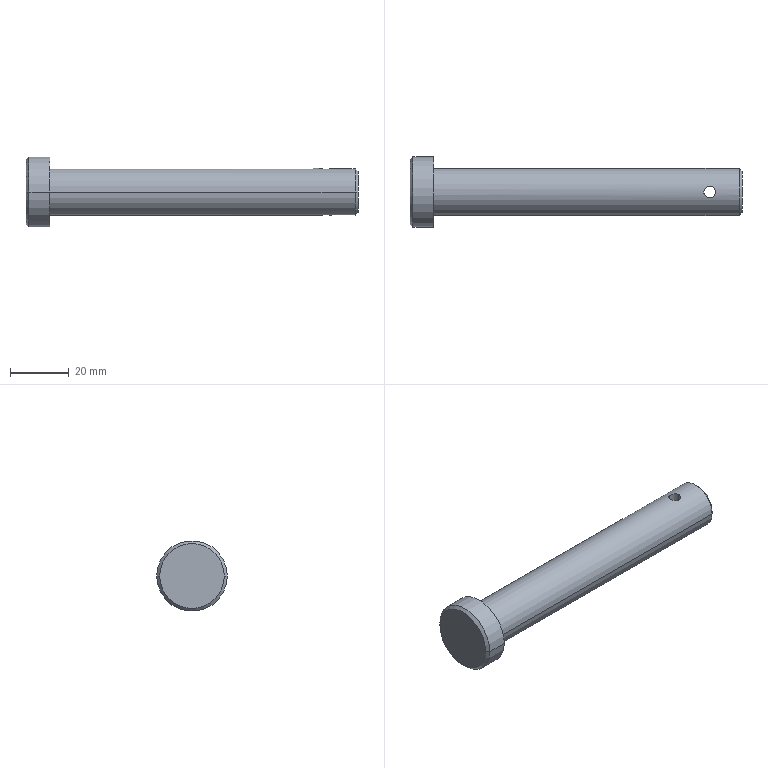Part | SolidWorks | features Chamfer 2, ICE 1, Revolution 1 | 1 solid | 13 faces | box 113 x 24 x 24 mm | volume 24470 mm3 | cylinder 6 | cone 4 | plane 3 | commonest cylinder face diameters 4 x2 16 x2 24 x2
STEP:
#1=CARTESIAN_POINT('',(-113.,-11.,0.));
#2=VERTEX_POINT('',#1);
#3=CARTESIAN_POINT('',(-113.,11.,0.));
#4=VERTEX_POINT('',#3);
#5=CARTESIAN_POINT('',(-113.,0.,0.));
#6=DIRECTION('',(-1.,0.,0.));
#7=DIRECTION('',(0.,-1.,0.));
#8=AXIS2_PLACEMENT_3D('',#5,#6,#7);
#9=CIRCLE('',#8,11.);
#10=EDGE_CURVE('',#2,#4,#9,.T.);
#11=ORIENTED_EDGE('',*,*,#10,.F.);
#12=CARTESIAN_POINT('',(-112.,-12.,0.));
#13=VERTEX_POINT('',#12);
#14=CARTESIAN_POINT('',(-112.,-12.,0.));
#15=DIRECTION('',(0.7071,-0.7071,0.));
#16=VECTOR('',#15,1000.);
#17=LINE('',#14,#16);
#18=EDGE_CURVE('',#2,#13,#17,.T.);
#19=ORIENTED_EDGE('',*,*,#18,.T.);
#20=CARTESIAN_POINT('',(-112.,12.,0.));
#21=VERTEX_POINT('',#20);
#22=CARTESIAN_POINT('',(-112.,0.,0.));
#23=DIRECTION('',(1.,0.,0.));
#24=DIRECTION('',(0.,-1.,0.));
#25=AXIS2_PLACEMENT_3D('',#22,#23,#24);
#26=CIRCLE('',#25,12.);
#27=EDGE_CURVE('',#21,#13,#26,.T.);
#28=ORIENTED_EDGE('',*,*,#27,.F.);
#29=CARTESIAN_POINT('',(-112.,12.,0.));
#30=DIRECTION('',(0.7071,0.7071,0.));
#31=VECTOR('',#30,1000.);
#32=LINE('',#29,#31);
#33=EDGE_CURVE('',#4,#21,#32,.T.);
#34=ORIENTED_EDGE('',*,*,#33,.F.);
#35=EDGE_LOOP('',(#11,#19,#28,#34));
#36=FACE_OUTER_BOUND('',#35,.T.);
#37=CARTESIAN_POINT('',(-112.,0.,0.));
#38=DIRECTION('',(1.,0.,0.));
#39=DIRECTION('',(0.,1.,0.));
#40=AXIS2_PLACEMENT_3D('',#37,#38,#39);
#41=CONICAL_SURFACE('',#40,12.,0.7854);
#42=ADVANCED_FACE('',(#36),#41,.T.);
#43=CARTESIAN_POINT('',(0.,7.,0.));
#44=VERTEX_POINT('',#43);
#45=CARTESIAN_POINT('',(0.,-7.,0.));
#46=VERTEX_POINT('',#45);
#47=CARTESIAN_POINT('',(0.,0.,0.));
#48=DIRECTION('',(1.,0.,0.));
#49=DIRECTION('',(0.,1.,0.));
#50=AXIS2_PLACEMENT_3D('',#47,#48,#49);
#51=CIRCLE('',#50,7.);
#52=EDGE_CURVE('',#44,#46,#51,.T.);
#53=ORIENTED_EDGE('',*,*,#52,.F.);
#54=CARTESIAN_POINT('',(-1.,8.,0.));
#55=VERTEX_POINT('',#54);
#56=CARTESIAN_POINT('',(0.,7.,0.));
#57=DIRECTION('',(-0.7071,0.7071,0.));
#58=VECTOR('',#57,1000.);
#59=LINE('',#56,#58);
#60=EDGE_CURVE('',#44,#55,#59,.T.);
#61=ORIENTED_EDGE('',*,*,#60,.T.);
#62=CARTESIAN_POINT('',(-1.,-8.,0.));
#63=VERTEX_POINT('',#62);
#64=CARTESIAN_POINT('',(-1.,0.,0.));
#65=DIRECTION('',(-1.,0.,0.));
#66=DIRECTION('',(0.,1.,0.));
#67=AXIS2_PLACEMENT_3D('',#64,#65,#66);
#68=CIRCLE('',#67,8.);
#69=EDGE_CURVE('',#63,#55,#68,.T.);
#70=ORIENTED_EDGE('',*,*,#69,.F.);
#71=CARTESIAN_POINT('',(0.,-7.,0.));
#72=DIRECTION('',(-0.7071,-0.7071,0.));
#73=VECTOR('',#72,1000.);
#74=LINE('',#71,#73);
#75=EDGE_CURVE('',#46,#63,#74,.T.);
#76=ORIENTED_EDGE('',*,*,#75,.F.);
#77=EDGE_LOOP('',(#53,#61,#70,#76));
#78=FACE_OUTER_BOUND('',#77,.T.);
#79=CARTESIAN_POINT('',(0.,0.,0.));
#80=DIRECTION('',(-1.,0.,0.));
#81=DIRECTION('',(0.,-1.,0.));
#82=AXIS2_PLACEMENT_3D('',#79,#80,#81);
#83=CONICAL_SURFACE('',#82,7.,0.7854);
#84=ADVANCED_FACE('',(#78),#83,.T.);
#85=CARTESIAN_POINT('',(-9.,0.,-8.));
#86=VERTEX_POINT('',#85);
#87=CARTESIAN_POINT('',(-13.,0.,-8.));
#88=VERTEX_POINT('',#87);
#89=CARTESIAN_POINT('',(-9.,0.,-8.));
#90=CARTESIAN_POINT('',(-9.,-0.1327,-8.));
#91=CARTESIAN_POINT('',(-9.013,-0.2631,-7.997));
#92=CARTESIAN_POINT('',(-9.064,-0.5195,-7.984));
#93=CARTESIAN_POINT('',(-9.103,-0.6468,-7.975));
#94=CARTESIAN_POINT('',(-9.204,-0.8888,-7.951));
#95=CARTESIAN_POINT('',(-9.265,-1.003,-7.938));
#96=CARTESIAN_POINT('',(-9.41,-1.22,-7.907));
#97=CARTESIAN_POINT('',(-9.494,-1.323,-7.89));
#98=CARTESIAN_POINT('',(-9.77,-1.598,-7.841));
#99=CARTESIAN_POINT('',(-9.992,-1.747,-7.808));
#100=CARTESIAN_POINT('',(-10.353,-1.897,-7.772));
#101=CARTESIAN_POINT('',(-10.48,-1.936,-7.762));
#102=CARTESIAN_POINT('',(-10.738,-1.987,-7.749));
#103=CARTESIAN_POINT('',(-10.868,-2.,-7.746));
#104=CARTESIAN_POINT('',(-11.13,-2.,-7.746));
#105=CARTESIAN_POINT('',(-11.263,-1.987,-7.749));
#106=CARTESIAN_POINT('',(-11.52,-1.936,-7.762));
#107=CARTESIAN_POINT('',(-11.645,-1.898,-7.772));
#108=CARTESIAN_POINT('',(-12.009,-1.746,-7.808));
#109=CARTESIAN_POINT('',(-12.229,-1.599,-7.841));
#110=CARTESIAN_POINT('',(-12.507,-1.321,-7.891));
#111=CARTESIAN_POINT('',(-12.59,-1.221,-7.907));
#112=CARTESIAN_POINT('',(-12.734,-1.005,-7.937));
#113=CARTESIAN_POINT('',(-12.797,-0.8874,-7.952));
#114=CARTESIAN_POINT('',(-12.897,-0.646,-7.975));
#115=CARTESIAN_POINT('',(-12.935,-0.5212,-7.984));
#116=CARTESIAN_POINT('',(-12.987,-0.2636,-7.997));
#117=CARTESIAN_POINT('',(-13.,-0.1308,-8.));
#118=CARTESIAN_POINT('',(-13.,0.,-8.));
#119=B_SPLINE_CURVE_WITH_KNOTS('',3,(#89,#90,#91,#92,#93,#94,#95,#96,#97,#98,#99,#100,#101,#102,#103,#104,#105,#106,#107,#108,#109,#110,#111,#112,#113,#114,#115,#116,#117,#118),.UNSPECIFIED.,.F.,.F.,(4,2,2,2,2,2,2,2,2,2,2,2,2,2,4),(0.,0.0003924,0.0007847,0.001177,0.001569,0.002354,0.002747,0.003139,0.003531,0.003924,0.004708,0.005101,0.005493,0.005886,0.006278),.UNSPECIFIED.);
#120=EDGE_CURVE('',#86,#88,#119,.T.);
#121=ORIENTED_EDGE('',*,*,#120,.T.);
#122=CARTESIAN_POINT('',(-13.,0.,8.));
#123=VERTEX_POINT('',#122);
#124=CARTESIAN_POINT('',(-13.,0.,-12.));
#125=DIRECTION('',(0.,0.,1.));
#126=VECTOR('',#125,1000.);
#127=LINE('',#124,#126);
#128=EDGE_CURVE('',#88,#123,#127,.T.);
#129=ORIENTED_EDGE('',*,*,#128,.T.);
#130=CARTESIAN_POINT('',(-9.,0.,8.));
#131=VERTEX_POINT('',#130);
#132=CARTESIAN_POINT('',(-13.,0.,8.));
#133=CARTESIAN_POINT('',(-13.,-0.2616,8.));
#134=CARTESIAN_POINT('',(-12.947,-0.5257,7.986));
#135=CARTESIAN_POINT('',(-12.797,-0.8871,7.952));
#136=CARTESIAN_POINT('',(-12.735,-1.004,7.937));
#137=CARTESIAN_POINT('',(-12.589,-1.221,7.907));
#138=CARTESIAN_POINT('',(-12.507,-1.321,7.891));
#139=CARTESIAN_POINT('',(-12.323,-1.506,7.858));
#140=CARTESIAN_POINT('',(-12.22,-1.59,7.841));
#141=CARTESIAN_POINT('',(-12.004,-1.734,7.81));
#142=CARTESIAN_POINT('',(-11.89,-1.796,7.796));
#143=CARTESIAN_POINT('',(-11.525,-1.948,7.76));
#144=CARTESIAN_POINT('',(-11.264,-2.,7.746));
#145=CARTESIAN_POINT('',(-10.869,-2.,7.746));
#146=CARTESIAN_POINT('',(-10.739,-1.987,7.749));
#147=CARTESIAN_POINT('',(-10.482,-1.936,7.762));
#148=CARTESIAN_POINT('',(-10.354,-1.897,7.772));
#149=CARTESIAN_POINT('',(-9.992,-1.747,7.808));
#150=CARTESIAN_POINT('',(-9.77,-1.598,7.841));
#151=CARTESIAN_POINT('',(-9.403,-1.232,7.907));
#152=CARTESIAN_POINT('',(-9.254,-1.01,7.94));
#153=CARTESIAN_POINT('',(-9.104,-0.6486,7.975));
#154=CARTESIAN_POINT('',(-9.065,-0.5212,7.984));
#155=CARTESIAN_POINT('',(-9.013,-0.2634,7.997));
#156=CARTESIAN_POINT('',(-9.,-0.1327,8.));
#157=CARTESIAN_POINT('',(-9.,0.,8.));
#158=B_SPLINE_CURVE_WITH_KNOTS('',3,(#132,#133,#134,#135,#136,#137,#138,#139,#140,#141,#142,#143,#144,#145,#146,#147,#148,#149,#150,#151,#152,#153,#154,#155,#156,#157),.UNSPECIFIED.,.F.,.F.,(4,2,2,2,2,2,2,2,2,2,2,2,4),(0.006278,0.007062,0.007455,0.007847,0.008239,0.008631,0.009416,0.009808,0.0102,0.01099,0.01177,0.01216,0.01255),.UNSPECIFIED.);
#159=EDGE_CURVE('',#123,#131,#158,.T.);
#160=ORIENTED_EDGE('',*,*,#159,.T.);
#161=CARTESIAN_POINT('',(-9.,0.,-12.));
#162=DIRECTION('',(0.,0.,1.));
#163=VECTOR('',#162,1000.);
#164=LINE('',#161,#163);
#165=EDGE_CURVE('',#86,#131,#164,.T.);
#166=ORIENTED_EDGE('',*,*,#165,.F.);
#167=EDGE_LOOP('',(#121,#129,#160,#166));
#168=FACE_OUTER_BOUND('',#167,.T.);
#169=CARTESIAN_POINT('',(-11.,0.,-12.));
#170=DIRECTION('',(0.,0.,1.));
#171=DIRECTION('',(1.,0.,0.));
#172=AXIS2_PLACEMENT_3D('',#169,#170,#171);
#173=CYLINDRICAL_SURFACE('',#172,2.);
#174=ADVANCED_FACE('',(#168),#173,.F.);
#175=CARTESIAN_POINT('',(-9.,0.,8.));
#176=CARTESIAN_POINT('',(-9.,0.1327,8.));
#177=CARTESIAN_POINT('',(-9.013,0.2631,7.997));
#178=CARTESIAN_POINT('',(-9.064,0.5195,7.984));
#179=CARTESIAN_POINT('',(-9.103,0.6468,7.975));
#180=CARTESIAN_POINT('',(-9.204,0.8888,7.951));
#181=CARTESIAN_POINT('',(-9.265,1.003,7.938));
#182=CARTESIAN_POINT('',(-9.41,1.22,7.907));
#183=CARTESIAN_POINT('',(-9.494,1.323,7.89));
#184=CARTESIAN_POINT('',(-9.77,1.598,7.841));
#185=CARTESIAN_POINT('',(-9.992,1.747,7.808));
#186=CARTESIAN_POINT('',(-10.353,1.897,7.772));
#187=CARTESIAN_POINT('',(-10.48,1.936,7.762));
#188=CARTESIAN_POINT('',(-10.738,1.987,7.749));
#189=CARTESIAN_POINT('',(-10.868,2.,7.746));
#190=CARTESIAN_POINT('',(-11.13,2.,7.746));
#191=CARTESIAN_POINT('',(-11.263,1.987,7.749));
#192=CARTESIAN_POINT('',(-11.52,1.936,7.762));
#193=CARTESIAN_POINT('',(-11.645,1.898,7.772));
#194=CARTESIAN_POINT('',(-12.009,1.746,7.808));
#195=CARTESIAN_POINT('',(-12.229,1.599,7.841));
#196=CARTESIAN_POINT('',(-12.507,1.321,7.891));
#197=CARTESIAN_POINT('',(-12.59,1.221,7.907));
#198=CARTESIAN_POINT('',(-12.734,1.005,7.937));
#199=CARTESIAN_POINT('',(-12.797,0.8874,7.952));
#200=CARTESIAN_POINT('',(-12.897,0.646,7.975));
#201=CARTESIAN_POINT('',(-12.935,0.5212,7.984));
#202=CARTESIAN_POINT('',(-12.987,0.2636,7.997));
#203=CARTESIAN_POINT('',(-13.,0.1308,8.));
#204=CARTESIAN_POINT('',(-13.,0.,8.));
#205=B_SPLINE_CURVE_WITH_KNOTS('',3,(#175,#176,#177,#178,#179,#180,#181,#182,#183,#184,#185,#186,#187,#188,#189,#190,#191,#192,#193,#194,#195,#196,#197,#198,#199,#200,#201,#202,#203,#204),.UNSPECIFIED.,.F.,.F.,(4,2,2,2,2,2,2,2,2,2,2,2,2,2,4),(0.,0.0003924,0.0007847,0.001177,0.001569,0.002354,0.002747,0.003139,0.003531,0.003924,0.004708,0.005101,0.005493,0.005886,0.006278),.UNSPECIFIED.);
#206=EDGE_CURVE('',#131,#123,#205,.T.);
#207=ORIENTED_EDGE('',*,*,#206,.F.);
#208=ORIENTED_EDGE('',*,*,#159,.F.);
#209=EDGE_LOOP('',(#207,#208));
#210=FACE_BOUND('',#209,.T.);
#211=CARTESIAN_POINT('',(-105.,8.,0.));
#212=VERTEX_POINT('',#211);
#213=CARTESIAN_POINT('',(-105.,-8.,0.));
#214=VERTEX_POINT('',#213);
#215=CARTESIAN_POINT('',(-105.,0.,0.));
#216=DIRECTION('',(1.,0.,0.));
#217=DIRECTION('',(0.,1.,0.));
#218=AXIS2_PLACEMENT_3D('',#215,#216,#217);
#219=CIRCLE('',#218,8.);
#220=EDGE_CURVE('',#212,#214,#219,.T.);
#221=ORIENTED_EDGE('',*,*,#220,.T.);
#222=CARTESIAN_POINT('',(0.,-8.,0.));
#223=DIRECTION('',(1.,0.,0.));
#224=VECTOR('',#223,1000.);
#225=LINE('',#222,#224);
#226=EDGE_CURVE('',#214,#63,#225,.T.);
#227=ORIENTED_EDGE('',*,*,#226,.T.);
#228=ORIENTED_EDGE('',*,*,#69,.T.);
#229=CARTESIAN_POINT('',(0.,8.,0.));
#230=DIRECTION('',(1.,0.,0.));
#231=VECTOR('',#230,1000.);
#232=LINE('',#229,#231);
#233=EDGE_CURVE('',#212,#55,#232,.T.);
#234=ORIENTED_EDGE('',*,*,#233,.F.);
#235=EDGE_LOOP('',(#221,#227,#228,#234));
#236=FACE_OUTER_BOUND('',#235,.T.);
#237=CARTESIAN_POINT('',(0.,0.,0.));
#238=DIRECTION('',(1.,0.,0.));
#239=DIRECTION('',(0.,1.,0.));
#240=AXIS2_PLACEMENT_3D('',#237,#238,#239);
#241=CYLINDRICAL_SURFACE('',#240,8.);
#242=ADVANCED_FACE('',(#210,#236),#241,.T.);
#243=ORIENTED_EDGE('',*,*,#27,.T.);
#244=CARTESIAN_POINT('',(-105.,-12.,0.));
#245=VERTEX_POINT('',#244);
#246=CARTESIAN_POINT('',(0.,-12.,0.));
#247=DIRECTION('',(1.,0.,0.));
#248=VECTOR('',#247,1000.);
#249=LINE('',#246,#248);
#250=EDGE_CURVE('',#13,#245,#249,.T.);
#251=ORIENTED_EDGE('',*,*,#250,.T.);
#252=CARTESIAN_POINT('',(-105.,12.,0.));
#253=VERTEX_POINT('',#252);
#254=CARTESIAN_POINT('',(-105.,0.,0.));
#255=DIRECTION('',(1.,0.,0.));
#256=DIRECTION('',(0.,1.,0.));
#257=AXIS2_PLACEMENT_3D('',#254,#255,#256);
#258=CIRCLE('',#257,12.);
#259=EDGE_CURVE('',#253,#245,#258,.T.);
#260=ORIENTED_EDGE('',*,*,#259,.F.);
#261=CARTESIAN_POINT('',(0.,12.,0.));
#262=DIRECTION('',(1.,0.,0.));
#263=VECTOR('',#262,1000.);
#264=LINE('',#261,#263);
#265=EDGE_CURVE('',#21,#253,#264,.T.);
#266=ORIENTED_EDGE('',*,*,#265,.F.);
#267=EDGE_LOOP('',(#243,#251,#260,#266));
#268=FACE_OUTER_BOUND('',#267,.T.);
#269=CARTESIAN_POINT('',(0.,0.,0.));
#270=DIRECTION('',(1.,0.,0.));
#271=DIRECTION('',(0.,1.,0.));
#272=AXIS2_PLACEMENT_3D('',#269,#270,#271);
#273=CYLINDRICAL_SURFACE('',#272,12.);
#274=ADVANCED_FACE('',(#268),#273,.T.);
#275=CARTESIAN_POINT('',(0.,0.,0.));
#276=DIRECTION('',(1.,0.,0.));
#277=DIRECTION('',(0.,1.,0.));
#278=AXIS2_PLACEMENT_3D('',#275,#276,#277);
#279=CIRCLE('',#278,7.);
#280=EDGE_CURVE('',#46,#44,#279,.T.);
#281=ORIENTED_EDGE('',*,*,#280,.T.);
#282=ORIENTED_EDGE('',*,*,#52,.T.);
#283=EDGE_LOOP('',(#281,#282));
#284=FACE_OUTER_BOUND('',#283,.T.);
#285=CARTESIAN_POINT('',(0.,8.,0.));
#286=DIRECTION('',(1.,0.,0.));
#287=DIRECTION('',(0.,1.,0.));
#288=AXIS2_PLACEMENT_3D('',#285,#286,#287);
#289=PLANE('',#288);
#290=ADVANCED_FACE('',(#284),#289,.T.);
#291=CARTESIAN_POINT('',(-113.,0.,0.));
#292=DIRECTION('',(-1.,0.,0.));
#293=DIRECTION('',(0.,-1.,0.));
#294=AXIS2_PLACEMENT_3D('',#291,#292,#293);
#295=CIRCLE('',#294,11.);
#296=EDGE_CURVE('',#4,#2,#295,.T.);
#297=ORIENTED_EDGE('',*,*,#296,.T.);
#298=ORIENTED_EDGE('',*,*,#10,.T.);
#299=EDGE_LOOP('',(#297,#298));
#300=FACE_OUTER_BOUND('',#299,.T.);
#301=CARTESIAN_POINT('',(-113.,0.,0.));
#302=DIRECTION('',(-1.,0.,0.));
#303=DIRECTION('',(0.,-1.,0.));
#304=AXIS2_PLACEMENT_3D('',#301,#302,#303);
#305=PLANE('',#304);
#306=ADVANCED_FACE('',(#300),#305,.T.);
#307=ORIENTED_EDGE('',*,*,#250,.F.);
#308=CARTESIAN_POINT('',(-112.,0.,0.));
#309=DIRECTION('',(1.,0.,0.));
#310=DIRECTION('',(0.,-1.,0.));
#311=AXIS2_PLACEMENT_3D('',#308,#309,#310);
#312=CIRCLE('',#311,12.);
#313=EDGE_CURVE('',#13,#21,#312,.T.);
#314=ORIENTED_EDGE('',*,*,#313,.T.);
#315=ORIENTED_EDGE('',*,*,#265,.T.);
#316=CARTESIAN_POINT('',(-105.,0.,0.));
#317=DIRECTION('',(1.,0.,0.));
#318=DIRECTION('',(0.,1.,0.));
#319=AXIS2_PLACEMENT_3D('',#316,#317,#318);
#320=CIRCLE('',#319,12.);
#321=EDGE_CURVE('',#245,#253,#320,.T.);
#322=ORIENTED_EDGE('',*,*,#321,.F.);
#323=EDGE_LOOP('',(#307,#314,#315,#322));
#324=FACE_OUTER_BOUND('',#323,.T.);
#325=CARTESIAN_POINT('',(0.,0.,0.));
#326=DIRECTION('',(1.,0.,0.));
#327=DIRECTION('',(0.,1.,0.));
#328=AXIS2_PLACEMENT_3D('',#325,#326,#327);
#329=CYLINDRICAL_SURFACE('',#328,12.);
#330=ADVANCED_FACE('',(#324),#329,.T.);
#331=ORIENTED_EDGE('',*,*,#259,.T.);
#332=ORIENTED_EDGE('',*,*,#321,.T.);
#333=EDGE_LOOP('',(#331,#332));
#334=FACE_OUTER_BOUND('',#333,.T.);
#335=ORIENTED_EDGE('',*,*,#220,.F.);
#336=CARTESIAN_POINT('',(-105.,0.,0.));
#337=DIRECTION('',(1.,0.,0.));
#338=DIRECTION('',(0.,1.,0.));
#339=AXIS2_PLACEMENT_3D('',#336,#337,#338);
#340=CIRCLE('',#339,8.);
#341=EDGE_CURVE('',#214,#212,#340,.T.);
#342=ORIENTED_EDGE('',*,*,#341,.F.);
#343=EDGE_LOOP('',(#335,#342));
#344=FACE_BOUND('',#343,.T.);
#345=CARTESIAN_POINT('',(-105.,12.,0.));
#346=DIRECTION('',(1.,0.,0.));
#347=DIRECTION('',(0.,1.,0.));
#348=AXIS2_PLACEMENT_3D('',#345,#346,#347);
#349=PLANE('',#348);
#350=ADVANCED_FACE('',(#334,#344),#349,.T.);
#351=ORIENTED_EDGE('',*,*,#226,.F.);
#352=ORIENTED_EDGE('',*,*,#341,.T.);
#353=ORIENTED_EDGE('',*,*,#233,.T.);
#354=CARTESIAN_POINT('',(-1.,0.,0.));
#355=DIRECTION('',(-1.,0.,0.));
#356=DIRECTION('',(0.,1.,0.));
#357=AXIS2_PLACEMENT_3D('',#354,#355,#356);
#358=CIRCLE('',#357,8.);
#359=EDGE_CURVE('',#55,#63,#358,.T.);
#360=ORIENTED_EDGE('',*,*,#359,.T.);
#361=EDGE_LOOP('',(#351,#352,#353,#360));
#362=FACE_OUTER_BOUND('',#361,.T.);
#363=ORIENTED_EDGE('',*,*,#120,.F.);
#364=CARTESIAN_POINT('',(-13.,0.,-8.));
#365=CARTESIAN_POINT('',(-13.,0.2616,-8.));
#366=CARTESIAN_POINT('',(-12.947,0.5257,-7.986));
#367=CARTESIAN_POINT('',(-12.797,0.8871,-7.952));
#368=CARTESIAN_POINT('',(-12.735,1.004,-7.937));
#369=CARTESIAN_POINT('',(-12.589,1.221,-7.907));
#370=CARTESIAN_POINT('',(-12.507,1.321,-7.891));
#371=CARTESIAN_POINT('',(-12.323,1.506,-7.858));
#372=CARTESIAN_POINT('',(-12.22,1.59,-7.841));
#373=CARTESIAN_POINT('',(-12.004,1.734,-7.81));
#374=CARTESIAN_POINT('',(-11.89,1.796,-7.796));
#375=CARTESIAN_POINT('',(-11.525,1.948,-7.76));
#376=CARTESIAN_POINT('',(-11.264,2.,-7.746));
#377=CARTESIAN_POINT('',(-10.869,2.,-7.746));
#378=CARTESIAN_POINT('',(-10.739,1.987,-7.749));
#379=CARTESIAN_POINT('',(-10.482,1.936,-7.762));
#380=CARTESIAN_POINT('',(-10.354,1.897,-7.772));
#381=CARTESIAN_POINT('',(-9.992,1.747,-7.808));
#382=CARTESIAN_POINT('',(-9.77,1.598,-7.841));
#383=CARTESIAN_POINT('',(-9.403,1.232,-7.907));
#384=CARTESIAN_POINT('',(-9.254,1.01,-7.94));
#385=CARTESIAN_POINT('',(-9.104,0.6486,-7.975));
#386=CARTESIAN_POINT('',(-9.065,0.5212,-7.984));
#387=CARTESIAN_POINT('',(-9.013,0.2634,-7.997));
#388=CARTESIAN_POINT('',(-9.,0.1327,-8.));
#389=CARTESIAN_POINT('',(-9.,0.,-8.));
#390=B_SPLINE_CURVE_WITH_KNOTS('',3,(#364,#365,#366,#367,#368,#369,#370,#371,#372,#373,#374,#375,#376,#377,#378,#379,#380,#381,#382,#383,#384,#385,#386,#387,#388,#389),.UNSPECIFIED.,.F.,.F.,(4,2,2,2,2,2,2,2,2,2,2,2,4),(0.006278,0.007062,0.007455,0.007847,0.008239,0.008631,0.009416,0.009808,0.0102,0.01099,0.01177,0.01216,0.01255),.UNSPECIFIED.);
#391=EDGE_CURVE('',#88,#86,#390,.T.);
#392=ORIENTED_EDGE('',*,*,#391,.F.);
#393=EDGE_LOOP('',(#363,#392));
#394=FACE_BOUND('',#393,.T.);
#395=CARTESIAN_POINT('',(0.,0.,0.));
#396=DIRECTION('',(1.,0.,0.));
#397=DIRECTION('',(0.,1.,0.));
#398=AXIS2_PLACEMENT_3D('',#395,#396,#397);
#399=CYLINDRICAL_SURFACE('',#398,8.);
#400=ADVANCED_FACE('',(#362,#394),#399,.T.);
#401=ORIENTED_EDGE('',*,*,#128,.F.);
#402=ORIENTED_EDGE('',*,*,#391,.T.);
#403=ORIENTED_EDGE('',*,*,#165,.T.);
#404=ORIENTED_EDGE('',*,*,#206,.T.);
#405=EDGE_LOOP('',(#401,#402,#403,#404));
#406=FACE_OUTER_BOUND('',#405,.T.);
#407=CARTESIAN_POINT('',(-11.,0.,-12.));
#408=DIRECTION('',(0.,0.,1.));
#409=DIRECTION('',(1.,0.,0.));
#410=AXIS2_PLACEMENT_3D('',#407,#408,#409);
#411=CYLINDRICAL_SURFACE('',#410,2.);
#412=ADVANCED_FACE('',(#406),#411,.F.);
#413=ORIENTED_EDGE('',*,*,#60,.F.);
#414=ORIENTED_EDGE('',*,*,#280,.F.);
#415=ORIENTED_EDGE('',*,*,#75,.T.);
#416=ORIENTED_EDGE('',*,*,#359,.F.);
#417=EDGE_LOOP('',(#413,#414,#415,#416));
#418=FACE_OUTER_BOUND('',#417,.T.);
#419=CARTESIAN_POINT('',(0.,0.,0.));
#420=DIRECTION('',(-1.,0.,0.));
#421=DIRECTION('',(0.,-1.,0.));
#422=AXIS2_PLACEMENT_3D('',#419,#420,#421);
#423=CONICAL_SURFACE('',#422,7.,0.7854);
#424=ADVANCED_FACE('',(#418),#423,.T.);
#425=ORIENTED_EDGE('',*,*,#18,.F.);
#426=ORIENTED_EDGE('',*,*,#296,.F.);
#427=ORIENTED_EDGE('',*,*,#33,.T.);
#428=ORIENTED_EDGE('',*,*,#313,.F.);
#429=EDGE_LOOP('',(#425,#426,#427,#428));
#430=FACE_OUTER_BOUND('',#429,.T.);
#431=CARTESIAN_POINT('',(-112.,0.,0.));
#432=DIRECTION('',(1.,0.,0.));
#433=DIRECTION('',(0.,1.,0.));
#434=AXIS2_PLACEMENT_3D('',#431,#432,#433);
#435=CONICAL_SURFACE('',#434,12.,0.7854);
#436=ADVANCED_FACE('',(#430),#435,.T.);
#437=CLOSED_SHELL('',(#42,#84,#174,#242,#274,#290,#306,#330,#350,#400,#412,#424,#436));
#438=MANIFOLD_SOLID_BREP('',#437);
#439=CARTESIAN_POINT('',(0.,0.,0.));
#440=DIRECTION('',(0.,0.,1.));
#441=DIRECTION('',(1.,0.,0.));
#442=AXIS2_PLACEMENT_3D('',#439,#440,#441);
#443=(LENGTH_UNIT()NAMED_UNIT(*)SI_UNIT(.MILLI.,.METRE.));
#444=UNCERTAINTY_MEASURE_WITH_UNIT(LENGTH_MEASURE(0.00001),#443,'','');
#445=(NAMED_UNIT(*)PLANE_ANGLE_UNIT()SI_UNIT($,.RADIAN.));
#446=(NAMED_UNIT(*)SI_UNIT($,.STERADIAN.)SOLID_ANGLE_UNIT());
#447=(GEOMETRIC_REPRESENTATION_CONTEXT(3)GLOBAL_UNCERTAINTY_ASSIGNED_CONTEXT((#444))GLOBAL_UNIT_ASSIGNED_CONTEXT((#443,#445,#446))REPRESENTATION_CONTEXT('',''));
#448=ADVANCED_BREP_SHAPE_REPRESENTATION('',(#438,#442),#447);